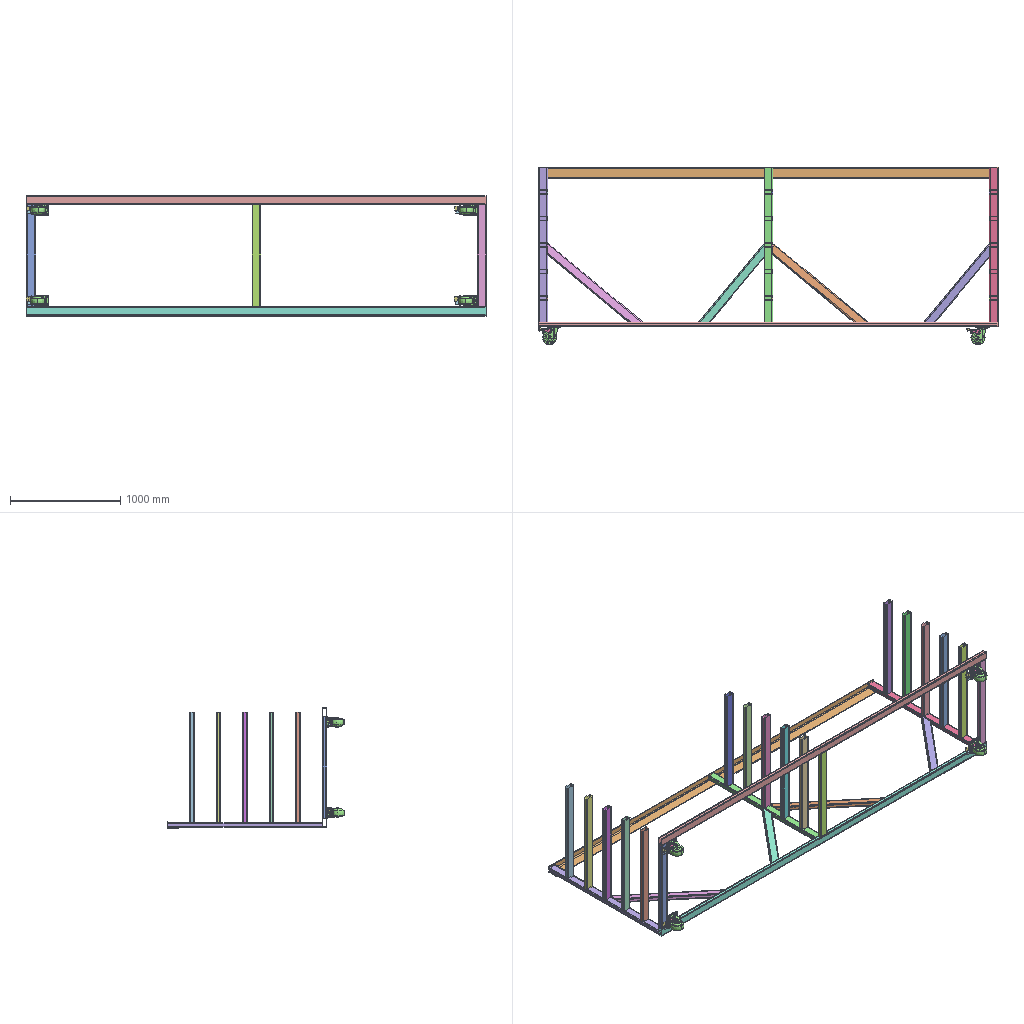Assembly | SolidWorks | 12 different items | 69 placed | box 4168 x 1610 x 1089 mm
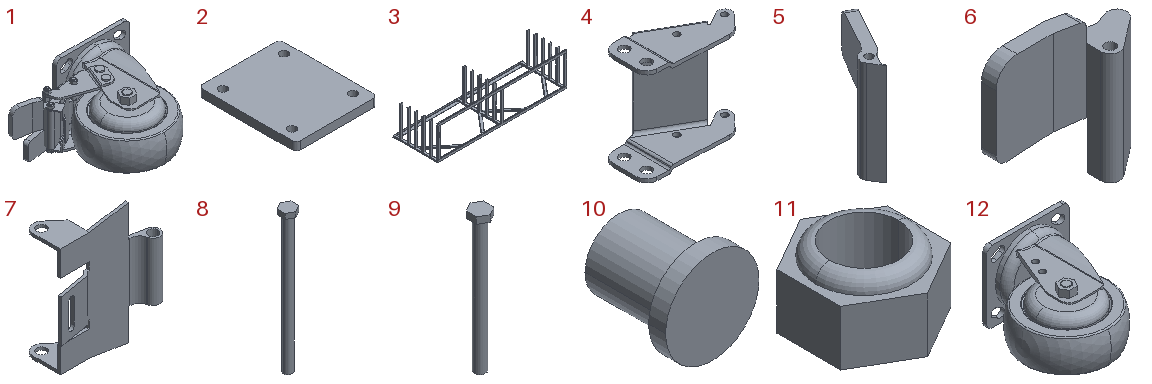Parts list (item | name | quantity | parent item | size | volume | features):
1 | (subassembly) | x4 | - | 202.75 x 164 x 100 mm | 915324 mm3 | -
2 | - | x4 | - | 100 x 120 x 10 mm | 116644 mm3 | features Extrusion 1
3 | - | x1 | - | 4160 x 1446 x 1089 mm | 33111474 mm3 | features WeldCornerFeat 7, 3DProfileFeature 2, MoveCopyBody 2, WeldMemberFeat 2, WeldmentFeature 1
4 | - | x4 | in 1 | 83.524 x 42.481 x 80.305 mm | 22865 mm3 | features BaseBody 1
5 | - | x4 | in 1 | 30.974 x 48.805 x 68 mm | 12607 mm3 | features BaseBody 1
6 | - | x4 | in 1 | 62.54 x 21.236 x 62 mm | 25261 mm3 | features BaseBody 1
7 | - | x4 | in 1 | 51.82 x 25.52 x 62.335 mm | 4576 mm3 | features BaseBody 1
8 | - | x8 | in 1 | 8 x 9.238 x 83.5 mm | 1745 mm3 | features BaseBody 1
9 | - | x4 | in 1 | 8 x 9.238 x 64.5 mm | 1372 mm3 | features BaseBody 1
10 | - | x16 | in 1 | 11 x 11 x 11 mm | 642.456 mm3 | features BaseBody 1
11 | - | x12 | in 1 | 8 x 9.238 x 5 mm | 157.594 mm3 | features BaseBody 1
12 | - | x4 | in 1 | 161.5 x 164 x 100 mm | 842029 mm3 | features BaseBody 1
Mates (type | each side: item.copy, entity, surface, feature):
Coincident | 3.1 face plane Rectangular tube 80 X 40 X 4.0(1) | 2.1 face plane Boss-Extrude1 | 2 times
DistanceDim | 2.1 face plane Boss-Extrude1 | 3.1 face plane Rectangular tube 80 X 40 X 4.0(1)
Coincident | 12.1 face plane Imported1 | 2.1 face plane Boss-Extrude1 | 3 times
Coincident | 3.1 face plane Rectangular tube 80 X 40 X 4.0(1) | 2.2 face plane Boss-Extrude1 | 3 times
Coincident | 12.2 face plane Imported1 | 2.2 face plane Boss-Extrude1 | 3 times
Coincident | 3.1 face plane Rectangular tube 80 X 40 X 4.0(1) | 2.3 face plane Boss-Extrude1 | 3 times
Coincident | 12.3 face plane Imported1 | 2.3 face plane Boss-Extrude1 | 3 times
Coincident | 3.1 face plane Rectangular tube 80 X 40 X 4.0(1) | 2.4 face plane Boss-Extrude1 | 3 times
Coincident | 12.4 face plane Imported1 | 2.4 face plane Boss-Extrude1 | 3 times